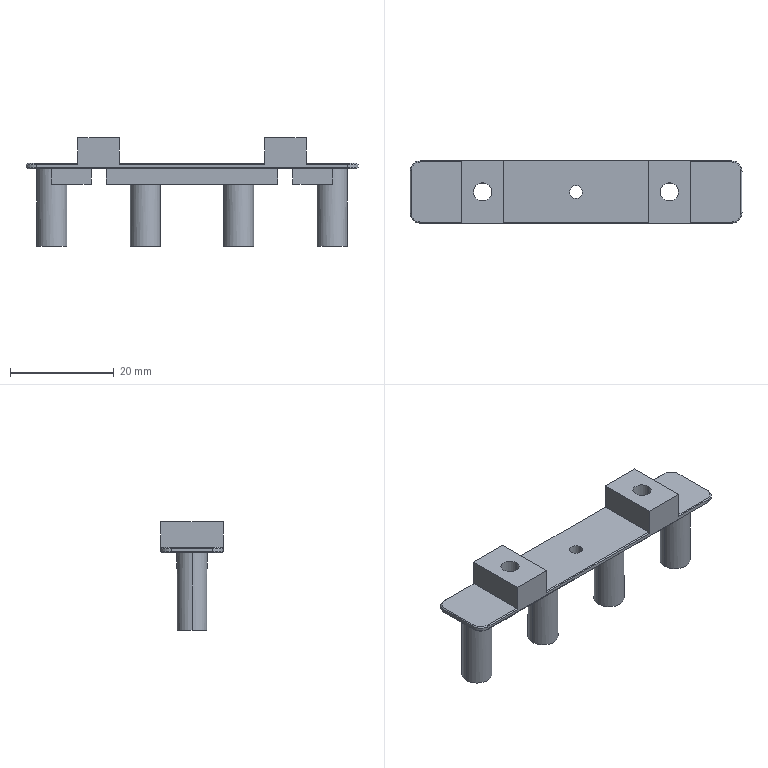NC program | NX | posted with a generic post | part box 64 x 12 x 21 mm
Lines 1 to 54 of 2110:
N10 G17 G21 G94 G90
(FLOOR_WALL , TOOL : D80)
N12 T19 M6
N14 G54
N16 G17 G0 G90 X-77. Y0. S6500 M3
N18 G43 Z30. H19
N20 Z3.
N22 G94 G1 Z0. F1500.
N24 X-74.
N26 X74.
N28 X77.
N30 Z3.
N32 G0 Z30.
N34 M5
(DRILLING , TOOL : D6A45)
N36 T01 M6
N38 G54
N40 G17 G0 G90 X-18. Y0. S5000 M3
N42 G43 Z30. H1
N44 G94 G81 G98 Z-1. F250. R3.
N46 X0.
N48 X18.
N50 G80
N52 G0 X18. Y0. Z30.
N54 M5
(DRILLING_COPY , TOOL : 3.5ZT)
N56 T07 M6
N58 G54
N60 G17 G0 G90 X-18. Y0. S1910 M3
N62 G43 Z30. H7
N64 G94 G73 G98 Z-8.552 F200. Q2. R3.
N66 X18.
N68 G80
N70 G0 X18. Y0. Z30.
N72 M5
(DRILLING_COPY_COPY , TOOL : 2.5ZT)
N74 T02 M6
N76 G54
N78 G17 G0 G90 X0. Y0. S2674 M3
N80 G43 Z30. H2
N82 G94 G73 G98 Z-11.251 F150. Q2. R3.
N84 G80
N86 G0 X0. Y0. Z30.
N88 M5